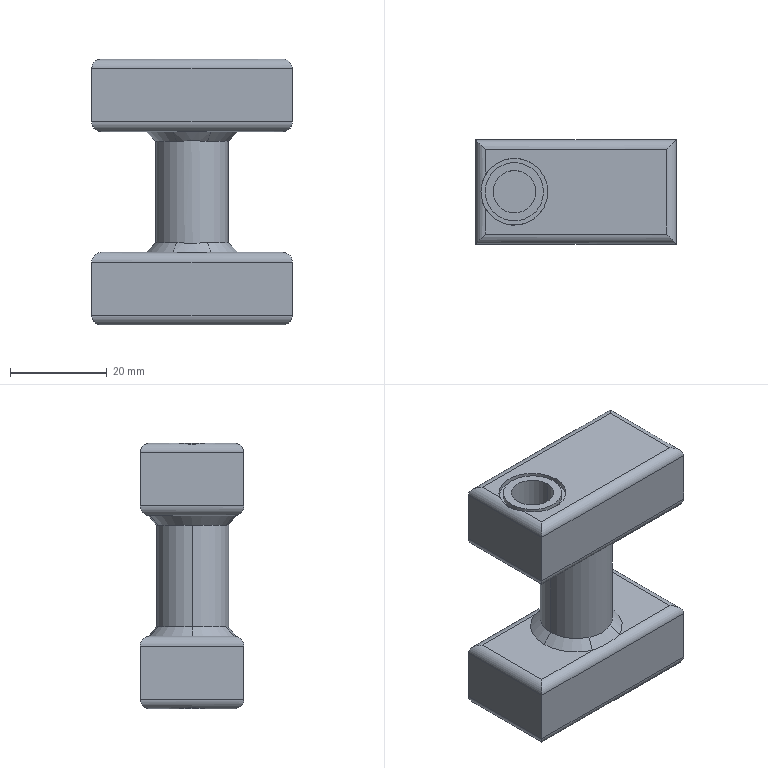Part | SolidWorks | features ICE 6, Chamfer 1, Extrusion 1, Fillet 1 | 1 solid | 60 faces | box 41.5 x 21.5 x 55 mm | volume 30038 mm3 | cylinder 30 | plane 20 | cone 6 | spline 4 | commonest cylinder face diameters 4 x16 8.8 x4 12.072 x4 13.852 x4 15 x2